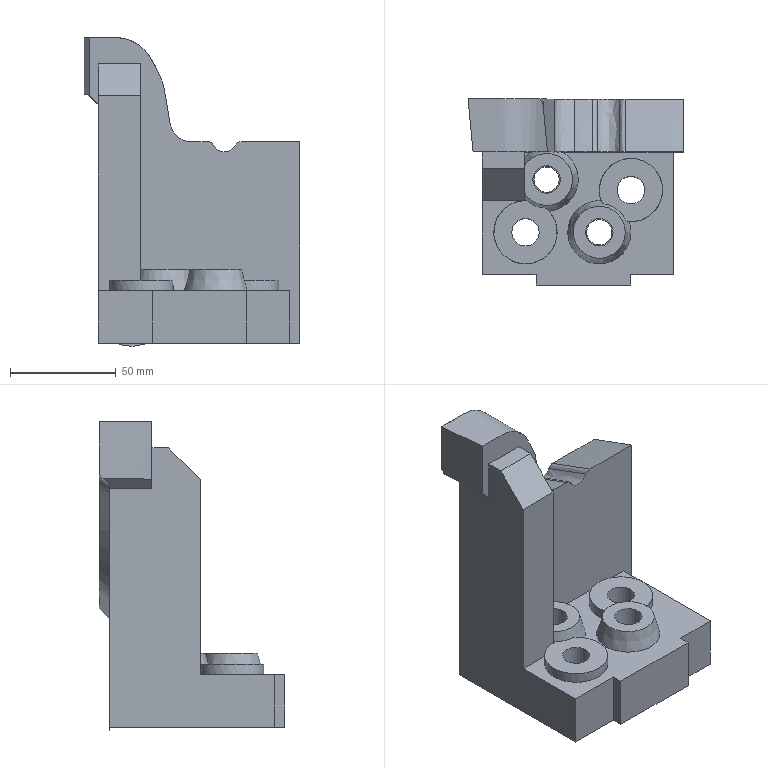Part | NX | features solid 2 | 1 solid | 49 faces | box 102.33 x 88.005 x 144.875 mm | volume 421435 mm3 | plane 25 | spline 14 | cylinder 8 | cone 2 | commonest cylinder face diameters 13 x4 12 x2 30 x2